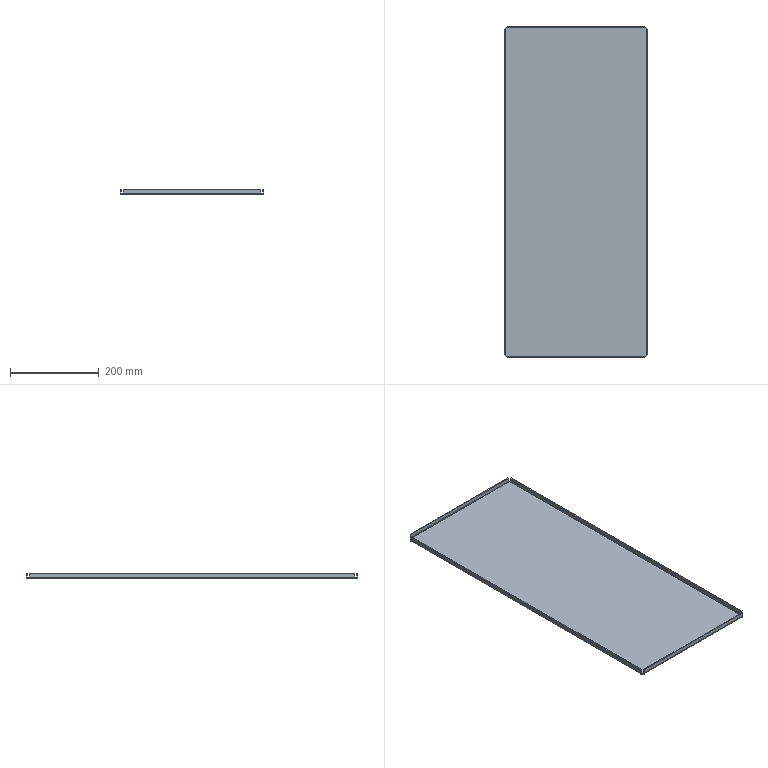Part | SolidWorks | features BaseBody 1 | 1 solid | 50 faces | box 325 x 750 x 12 mm | volume 654399 mm3 | plane 42 | cylinder 8 | commonest cylinder face diameters 1.473 x4 6.473 x4
STEP:
#1=CARTESIAN_POINT('',(-155.5,372.5,9.5));
#2=VERTEX_POINT('',#1);
#3=CARTESIAN_POINT('',(155.5,372.5,9.5));
#4=VERTEX_POINT('',#3);
#5=CARTESIAN_POINT('',(155.5,372.5,9.5));
#6=DIRECTION('',(1.,0.,0.));
#7=VECTOR('',#6,1000.);
#8=LINE('',#5,#7);
#9=EDGE_CURVE('',#2,#4,#8,.T.);
#10=ORIENTED_EDGE('',*,*,#9,.T.);
#11=CARTESIAN_POINT('',(155.5,375.,9.5));
#12=VERTEX_POINT('',#11);
#13=CARTESIAN_POINT('',(155.5,375.,9.5));
#14=DIRECTION('',(0.,-1.,0.));
#15=VECTOR('',#14,1000.);
#16=LINE('',#13,#15);
#17=EDGE_CURVE('',#12,#4,#16,.T.);
#18=ORIENTED_EDGE('',*,*,#17,.F.);
#19=CARTESIAN_POINT('',(-155.5,375.,9.5));
#20=VERTEX_POINT('',#19);
#21=CARTESIAN_POINT('',(0.,375.,9.5));
#22=DIRECTION('',(1.,0.,0.));
#23=VECTOR('',#22,1000.);
#24=LINE('',#21,#23);
#25=EDGE_CURVE('',#20,#12,#24,.T.);
#26=ORIENTED_EDGE('',*,*,#25,.F.);
#27=CARTESIAN_POINT('',(-155.5,375.,9.5));
#28=DIRECTION('',(0.,-1.,0.));
#29=VECTOR('',#28,1000.);
#30=LINE('',#27,#29);
#31=EDGE_CURVE('',#20,#2,#30,.T.);
#32=ORIENTED_EDGE('',*,*,#31,.T.);
#33=EDGE_LOOP('',(#10,#18,#26,#32));
#34=FACE_OUTER_BOUND('',#33,.T.);
#35=CARTESIAN_POINT('',(155.5,375.,9.5));
#36=DIRECTION('',(0.,0.,-1.));
#37=DIRECTION('',(0.,-1.,0.));
#38=AXIS2_PLACEMENT_3D('',#35,#36,#37);
#39=PLANE('',#38);
#40=ADVANCED_FACE('',(#34),#39,.F.);
#41=CARTESIAN_POINT('',(-155.5,372.5,0.7366));
#42=VERTEX_POINT('',#41);
#43=CARTESIAN_POINT('',(-155.5,372.5,9.5));
#44=DIRECTION('',(0.,0.,1.));
#45=VECTOR('',#44,1000.);
#46=LINE('',#43,#45);
#47=EDGE_CURVE('',#42,#2,#46,.T.);
#48=ORIENTED_EDGE('',*,*,#47,.F.);
#49=CARTESIAN_POINT('',(155.5,372.5,0.7366));
#50=VERTEX_POINT('',#49);
#51=CARTESIAN_POINT('',(155.5,372.5,0.7366));
#52=DIRECTION('',(-1.,0.,0.));
#53=VECTOR('',#52,1000.);
#54=LINE('',#51,#53);
#55=EDGE_CURVE('',#50,#42,#54,.T.);
#56=ORIENTED_EDGE('',*,*,#55,.F.);
#57=CARTESIAN_POINT('',(155.5,372.5,0.));
#58=DIRECTION('',(0.,0.,-1.));
#59=VECTOR('',#58,1000.);
#60=LINE('',#57,#59);
#61=EDGE_CURVE('',#4,#50,#60,.T.);
#62=ORIENTED_EDGE('',*,*,#61,.F.);
#63=ORIENTED_EDGE('',*,*,#9,.F.);
#64=EDGE_LOOP('',(#48,#56,#62,#63));
#65=FACE_OUTER_BOUND('',#64,.T.);
#66=CARTESIAN_POINT('',(0.,372.5,0.));
#67=DIRECTION('',(0.,-1.,0.));
#68=DIRECTION('',(-1.,0.,0.));
#69=AXIS2_PLACEMENT_3D('',#66,#67,#68);
#70=PLANE('',#69);
#71=ADVANCED_FACE('',(#65),#70,.T.);
#72=CARTESIAN_POINT('',(-155.5,375.,0.7366));
#73=VERTEX_POINT('',#72);
#74=CARTESIAN_POINT('',(155.5,375.,0.7366));
#75=VERTEX_POINT('',#74);
#76=CARTESIAN_POINT('',(155.5,375.,0.7366));
#77=DIRECTION('',(1.,0.,0.));
#78=VECTOR('',#77,1000.);
#79=LINE('',#76,#78);
#80=EDGE_CURVE('',#73,#75,#79,.T.);
#81=ORIENTED_EDGE('',*,*,#80,.F.);
#82=CARTESIAN_POINT('',(-155.5,375.,0.));
#83=DIRECTION('',(0.,0.,1.));
#84=VECTOR('',#83,1000.);
#85=LINE('',#82,#84);
#86=EDGE_CURVE('',#73,#20,#85,.T.);
#87=ORIENTED_EDGE('',*,*,#86,.T.);
#88=ORIENTED_EDGE('',*,*,#25,.T.);
#89=CARTESIAN_POINT('',(155.5,375.,0.));
#90=DIRECTION('',(0.,0.,-1.));
#91=VECTOR('',#90,1000.);
#92=LINE('',#89,#91);
#93=EDGE_CURVE('',#12,#75,#92,.T.);
#94=ORIENTED_EDGE('',*,*,#93,.T.);
#95=EDGE_LOOP('',(#81,#87,#88,#94));
#96=FACE_OUTER_BOUND('',#95,.T.);
#97=CARTESIAN_POINT('',(0.,375.,0.));
#98=DIRECTION('',(0.,-1.,0.));
#99=DIRECTION('',(-1.,0.,0.));
#100=AXIS2_PLACEMENT_3D('',#97,#98,#99);
#101=PLANE('',#100);
#102=ADVANCED_FACE('',(#96),#101,.F.);
#103=CARTESIAN_POINT('',(-155.5,372.5,0.7366));
#104=DIRECTION('',(0.,1.,0.));
#105=VECTOR('',#104,1000.);
#106=LINE('',#103,#105);
#107=EDGE_CURVE('',#42,#73,#106,.T.);
#108=ORIENTED_EDGE('',*,*,#107,.F.);
#109=ORIENTED_EDGE('',*,*,#47,.T.);
#110=ORIENTED_EDGE('',*,*,#31,.F.);
#111=ORIENTED_EDGE('',*,*,#86,.F.);
#112=EDGE_LOOP('',(#108,#109,#110,#111));
#113=FACE_OUTER_BOUND('',#112,.T.);
#114=CARTESIAN_POINT('',(-155.5,375.,9.5));
#115=DIRECTION('',(1.,0.,0.));
#116=DIRECTION('',(0.,0.,-1.));
#117=AXIS2_PLACEMENT_3D('',#114,#115,#116);
#118=PLANE('',#117);
#119=ADVANCED_FACE('',(#113),#118,.F.);
#120=CARTESIAN_POINT('',(155.5,375.,0.7366));
#121=DIRECTION('',(0.,1.,0.));
#122=VECTOR('',#121,1000.);
#123=LINE('',#120,#122);
#124=EDGE_CURVE('',#50,#75,#123,.T.);
#125=ORIENTED_EDGE('',*,*,#124,.T.);
#126=ORIENTED_EDGE('',*,*,#93,.F.);
#127=ORIENTED_EDGE('',*,*,#17,.T.);
#128=ORIENTED_EDGE('',*,*,#61,.T.);
#129=EDGE_LOOP('',(#125,#126,#127,#128));
#130=FACE_OUTER_BOUND('',#129,.T.);
#131=CARTESIAN_POINT('',(155.5,375.,0.));
#132=DIRECTION('',(-1.,0.,0.));
#133=DIRECTION('',(0.,1.,0.));
#134=AXIS2_PLACEMENT_3D('',#131,#132,#133);
#135=PLANE('',#134);
#136=ADVANCED_FACE('',(#130),#135,.F.);
#137=CARTESIAN_POINT('',(-155.5,371.763,0.));
#138=VERTEX_POINT('',#137);
#139=CARTESIAN_POINT('',(155.5,371.763,0.));
#140=VERTEX_POINT('',#139);
#141=CARTESIAN_POINT('',(-155.5,371.763,0.));
#142=DIRECTION('',(1.,0.,0.));
#143=VECTOR('',#142,1000.);
#144=LINE('',#141,#143);
#145=EDGE_CURVE('',#138,#140,#144,.T.);
#146=ORIENTED_EDGE('',*,*,#145,.T.);
#147=CARTESIAN_POINT('',(155.5,371.763,0.7366));
#148=DIRECTION('',(1.,0.,0.));
#149=DIRECTION('',(0.,0.,1.));
#150=AXIS2_PLACEMENT_3D('',#147,#148,#149);
#151=CIRCLE('',#150,0.7366);
#152=EDGE_CURVE('',#140,#50,#151,.T.);
#153=ORIENTED_EDGE('',*,*,#152,.T.);
#154=ORIENTED_EDGE('',*,*,#55,.T.);
#155=CARTESIAN_POINT('',(-155.5,371.763,0.7366));
#156=DIRECTION('',(-1.,0.,0.));
#157=DIRECTION('',(0.,0.,1.));
#158=AXIS2_PLACEMENT_3D('',#155,#156,#157);
#159=CIRCLE('',#158,0.7366);
#160=EDGE_CURVE('',#42,#138,#159,.T.);
#161=ORIENTED_EDGE('',*,*,#160,.T.);
#162=EDGE_LOOP('',(#146,#153,#154,#161));
#163=FACE_OUTER_BOUND('',#162,.T.);
#164=CARTESIAN_POINT('',(-155.5,371.763,0.7366));
#165=DIRECTION('',(-1.,0.,0.));
#166=DIRECTION('',(0.,1.,0.));
#167=AXIS2_PLACEMENT_3D('',#164,#165,#166);
#168=CYLINDRICAL_SURFACE('',#167,0.7366);
#169=ADVANCED_FACE('',(#163),#168,.F.);
#170=CARTESIAN_POINT('',(-155.5,371.763,-2.5));
#171=VERTEX_POINT('',#170);
#172=CARTESIAN_POINT('',(155.5,371.763,-2.5));
#173=VERTEX_POINT('',#172);
#174=CARTESIAN_POINT('',(-155.5,371.763,-2.5));
#175=DIRECTION('',(1.,0.,0.));
#176=VECTOR('',#175,1000.);
#177=LINE('',#174,#176);
#178=EDGE_CURVE('',#171,#173,#177,.T.);
#179=ORIENTED_EDGE('',*,*,#178,.F.);
#180=CARTESIAN_POINT('',(-155.5,374.915,0.));
#181=VERTEX_POINT('',#180);
#182=CARTESIAN_POINT('',(-155.5,371.763,0.7366));
#183=DIRECTION('',(-1.,0.,0.));
#184=DIRECTION('',(0.,0.,1.));
#185=AXIS2_PLACEMENT_3D('',#182,#183,#184);
#186=CIRCLE('',#185,3.237);
#187=EDGE_CURVE('',#181,#171,#186,.T.);
#188=ORIENTED_EDGE('',*,*,#187,.F.);
#189=CARTESIAN_POINT('',(-155.5,371.763,0.7366));
#190=DIRECTION('',(-1.,0.,0.));
#191=DIRECTION('',(0.,0.,1.));
#192=AXIS2_PLACEMENT_3D('',#189,#190,#191);
#193=CIRCLE('',#192,3.237);
#194=EDGE_CURVE('',#73,#181,#193,.T.);
#195=ORIENTED_EDGE('',*,*,#194,.F.);
#196=ORIENTED_EDGE('',*,*,#80,.T.);
#197=CARTESIAN_POINT('',(155.5,374.915,0.));
#198=VERTEX_POINT('',#197);
#199=CARTESIAN_POINT('',(155.5,371.763,0.7366));
#200=DIRECTION('',(1.,0.,0.));
#201=DIRECTION('',(0.,0.,1.));
#202=AXIS2_PLACEMENT_3D('',#199,#200,#201);
#203=CIRCLE('',#202,3.237);
#204=EDGE_CURVE('',#198,#75,#203,.T.);
#205=ORIENTED_EDGE('',*,*,#204,.F.);
#206=CARTESIAN_POINT('',(155.5,371.763,0.7366));
#207=DIRECTION('',(1.,0.,0.));
#208=DIRECTION('',(0.,0.,1.));
#209=AXIS2_PLACEMENT_3D('',#206,#207,#208);
#210=CIRCLE('',#209,3.237);
#211=EDGE_CURVE('',#173,#198,#210,.T.);
#212=ORIENTED_EDGE('',*,*,#211,.F.);
#213=EDGE_LOOP('',(#179,#188,#195,#196,#205,#212));
#214=FACE_OUTER_BOUND('',#213,.T.);
#215=CARTESIAN_POINT('',(-155.5,371.763,0.7366));
#216=DIRECTION('',(-1.,0.,0.));
#217=DIRECTION('',(0.,1.,0.));
#218=AXIS2_PLACEMENT_3D('',#215,#216,#217);
#219=CYLINDRICAL_SURFACE('',#218,3.237);
#220=ADVANCED_FACE('',(#214),#219,.T.);
#221=ORIENTED_EDGE('',*,*,#194,.T.);
#222=CARTESIAN_POINT('',(-155.5,375.,0.));
#223=DIRECTION('',(0.,-1.,0.));
#224=VECTOR('',#223,1000.);
#225=LINE('',#222,#224);
#226=EDGE_CURVE('',#181,#138,#225,.T.);
#227=ORIENTED_EDGE('',*,*,#226,.T.);
#228=ORIENTED_EDGE('',*,*,#160,.F.);
#229=ORIENTED_EDGE('',*,*,#107,.T.);
#230=EDGE_LOOP('',(#221,#227,#228,#229));
#231=FACE_OUTER_BOUND('',#230,.T.);
#232=CARTESIAN_POINT('',(-155.5,371.763,0.7366));
#233=DIRECTION('',(1.,0.,0.));
#234=DIRECTION('',(0.,1.,0.));
#235=AXIS2_PLACEMENT_3D('',#232,#233,#234);
#236=PLANE('',#235);
#237=ADVANCED_FACE('',(#231),#236,.F.);
#238=ORIENTED_EDGE('',*,*,#152,.F.);
#239=CARTESIAN_POINT('',(155.5,371.763,0.));
#240=DIRECTION('',(0.,1.,0.));
#241=VECTOR('',#240,1000.);
#242=LINE('',#239,#241);
#243=EDGE_CURVE('',#140,#198,#242,.T.);
#244=ORIENTED_EDGE('',*,*,#243,.T.);
#245=ORIENTED_EDGE('',*,*,#204,.T.);
#246=ORIENTED_EDGE('',*,*,#124,.F.);
#247=EDGE_LOOP('',(#238,#244,#245,#246));
#248=FACE_OUTER_BOUND('',#247,.T.);
#249=CARTESIAN_POINT('',(155.5,371.763,0.7366));
#250=DIRECTION('',(1.,0.,0.));
#251=DIRECTION('',(0.,1.,0.));
#252=AXIS2_PLACEMENT_3D('',#249,#250,#251);
#253=PLANE('',#252);
#254=ADVANCED_FACE('',(#248),#253,.T.);
#255=CARTESIAN_POINT('',(160.,368.,9.5));
#256=VERTEX_POINT('',#255);
#257=CARTESIAN_POINT('',(160.,-368.,9.5));
#258=VERTEX_POINT('',#257);
#259=CARTESIAN_POINT('',(160.,-368.,9.5));
#260=DIRECTION('',(0.,-1.,0.));
#261=VECTOR('',#260,1000.);
#262=LINE('',#259,#261);
#263=EDGE_CURVE('',#256,#258,#262,.T.);
#264=ORIENTED_EDGE('',*,*,#263,.T.);
#265=CARTESIAN_POINT('',(162.5,-368.,9.5));
#266=VERTEX_POINT('',#265);
#267=CARTESIAN_POINT('',(162.5,-368.,9.5));
#268=DIRECTION('',(-1.,0.,0.));
#269=VECTOR('',#268,1000.);
#270=LINE('',#267,#269);
#271=EDGE_CURVE('',#266,#258,#270,.T.);
#272=ORIENTED_EDGE('',*,*,#271,.F.);
#273=CARTESIAN_POINT('',(162.5,368.,9.5));
#274=VERTEX_POINT('',#273);
#275=CARTESIAN_POINT('',(162.5,0.,9.5));
#276=DIRECTION('',(0.,-1.,0.));
#277=VECTOR('',#276,1000.);
#278=LINE('',#275,#277);
#279=EDGE_CURVE('',#274,#266,#278,.T.);
#280=ORIENTED_EDGE('',*,*,#279,.F.);
#281=CARTESIAN_POINT('',(162.5,368.,9.5));
#282=DIRECTION('',(-1.,0.,0.));
#283=VECTOR('',#282,1000.);
#284=LINE('',#281,#283);
#285=EDGE_CURVE('',#274,#256,#284,.T.);
#286=ORIENTED_EDGE('',*,*,#285,.T.);
#287=EDGE_LOOP('',(#264,#272,#280,#286));
#288=FACE_OUTER_BOUND('',#287,.T.);
#289=CARTESIAN_POINT('',(162.5,-368.,9.5));
#290=DIRECTION('',(0.,0.,-1.));
#291=DIRECTION('',(-1.,0.,0.));
#292=AXIS2_PLACEMENT_3D('',#289,#290,#291);
#293=PLANE('',#292);
#294=ADVANCED_FACE('',(#288),#293,.F.);
#295=CARTESIAN_POINT('',(160.,368.,0.7366));
#296=VERTEX_POINT('',#295);
#297=CARTESIAN_POINT('',(160.,368.,9.5));
#298=DIRECTION('',(0.,0.,1.));
#299=VECTOR('',#298,1000.);
#300=LINE('',#297,#299);
#301=EDGE_CURVE('',#296,#256,#300,.T.);
#302=ORIENTED_EDGE('',*,*,#301,.F.);
#303=CARTESIAN_POINT('',(160.,-368.,0.7366));
#304=VERTEX_POINT('',#303);
#305=CARTESIAN_POINT('',(160.,-368.,0.7366));
#306=DIRECTION('',(0.,1.,0.));
#307=VECTOR('',#306,1000.);
#308=LINE('',#305,#307);
#309=EDGE_CURVE('',#304,#296,#308,.T.);
#310=ORIENTED_EDGE('',*,*,#309,.F.);
#311=CARTESIAN_POINT('',(160.,-368.,0.));
#312=DIRECTION('',(0.,0.,-1.));
#313=VECTOR('',#312,1000.);
#314=LINE('',#311,#313);
#315=EDGE_CURVE('',#258,#304,#314,.T.);
#316=ORIENTED_EDGE('',*,*,#315,.F.);
#317=ORIENTED_EDGE('',*,*,#263,.F.);
#318=EDGE_LOOP('',(#302,#310,#316,#317));
#319=FACE_OUTER_BOUND('',#318,.T.);
#320=CARTESIAN_POINT('',(160.,0.,0.));
#321=DIRECTION('',(-1.,0.,0.));
#322=DIRECTION('',(0.,1.,0.));
#323=AXIS2_PLACEMENT_3D('',#320,#321,#322);
#324=PLANE('',#323);
#325=ADVANCED_FACE('',(#319),#324,.T.);
#326=CARTESIAN_POINT('',(162.5,368.,0.7366));
#327=VERTEX_POINT('',#326);
#328=CARTESIAN_POINT('',(162.5,-368.,0.7366));
#329=VERTEX_POINT('',#328);
#330=CARTESIAN_POINT('',(162.5,-368.,0.7366));
#331=DIRECTION('',(0.,-1.,0.));
#332=VECTOR('',#331,1000.);
#333=LINE('',#330,#332);
#334=EDGE_CURVE('',#327,#329,#333,.T.);
#335=ORIENTED_EDGE('',*,*,#334,.F.);
#336=CARTESIAN_POINT('',(162.5,368.,0.));
#337=DIRECTION('',(0.,0.,1.));
#338=VECTOR('',#337,1000.);
#339=LINE('',#336,#338);
#340=EDGE_CURVE('',#327,#274,#339,.T.);
#341=ORIENTED_EDGE('',*,*,#340,.T.);
#342=ORIENTED_EDGE('',*,*,#279,.T.);
#343=CARTESIAN_POINT('',(162.5,-368.,0.));
#344=DIRECTION('',(0.,0.,-1.));
#345=VECTOR('',#344,1000.);
#346=LINE('',#343,#345);
#347=EDGE_CURVE('',#266,#329,#346,.T.);
#348=ORIENTED_EDGE('',*,*,#347,.T.);
#349=EDGE_LOOP('',(#335,#341,#342,#348));
#350=FACE_OUTER_BOUND('',#349,.T.);
#351=CARTESIAN_POINT('',(162.5,0.,0.));
#352=DIRECTION('',(-1.,0.,0.));
#353=DIRECTION('',(0.,1.,0.));
#354=AXIS2_PLACEMENT_3D('',#351,#352,#353);
#355=PLANE('',#354);
#356=ADVANCED_FACE('',(#350),#355,.F.);
#357=CARTESIAN_POINT('',(160.,368.,0.7366));
#358=DIRECTION('',(1.,0.,0.));
#359=VECTOR('',#358,1000.);
#360=LINE('',#357,#359);
#361=EDGE_CURVE('',#296,#327,#360,.T.);
#362=ORIENTED_EDGE('',*,*,#361,.F.);
#363=ORIENTED_EDGE('',*,*,#301,.T.);
#364=ORIENTED_EDGE('',*,*,#285,.F.);
#365=ORIENTED_EDGE('',*,*,#340,.F.);
#366=EDGE_LOOP('',(#362,#363,#364,#365));
#367=FACE_OUTER_BOUND('',#366,.T.);
#368=CARTESIAN_POINT('',(162.5,368.,9.5));
#369=DIRECTION('',(0.,-1.,0.));
#370=DIRECTION('',(0.,0.,-1.));
#371=AXIS2_PLACEMENT_3D('',#368,#369,#370);
#372=PLANE('',#371);
#373=ADVANCED_FACE('',(#367),#372,.F.);
#374=CARTESIAN_POINT('',(162.5,-368.,0.7366));
#375=DIRECTION('',(1.,0.,0.));
#376=VECTOR('',#375,1000.);
#377=LINE('',#374,#376);
#378=EDGE_CURVE('',#304,#329,#377,.T.);
#379=ORIENTED_EDGE('',*,*,#378,.T.);
#380=ORIENTED_EDGE('',*,*,#347,.F.);
#381=ORIENTED_EDGE('',*,*,#271,.T.);
#382=ORIENTED_EDGE('',*,*,#315,.T.);
#383=EDGE_LOOP('',(#379,#380,#381,#382));
#384=FACE_OUTER_BOUND('',#383,.T.);
#385=CARTESIAN_POINT('',(162.5,-368.,0.));
#386=DIRECTION('',(0.,1.,0.));
#387=DIRECTION('',(1.,0.,0.));
#388=AXIS2_PLACEMENT_3D('',#385,#386,#387);
#389=PLANE('',#388);
#390=ADVANCED_FACE('',(#384),#389,.F.);
#391=CARTESIAN_POINT('',(159.263,368.,0.));
#392=VERTEX_POINT('',#391);
#393=CARTESIAN_POINT('',(159.263,-368.,0.));
#394=VERTEX_POINT('',#393);
#395=CARTESIAN_POINT('',(159.263,368.,0.));
#396=DIRECTION('',(0.,-1.,0.));
#397=VECTOR('',#396,1000.);
#398=LINE('',#395,#397);
#399=EDGE_CURVE('',#392,#394,#398,.T.);
#400=ORIENTED_EDGE('',*,*,#399,.T.);
#401=CARTESIAN_POINT('',(159.263,-368.,0.7366));
#402=DIRECTION('',(0.,-1.,0.));
#403=DIRECTION('',(0.,0.,1.));
#404=AXIS2_PLACEMENT_3D('',#401,#402,#403);
#405=CIRCLE('',#404,0.7366);
#406=EDGE_CURVE('',#394,#304,#405,.T.);
#407=ORIENTED_EDGE('',*,*,#406,.T.);
#408=ORIENTED_EDGE('',*,*,#309,.T.);
#409=CARTESIAN_POINT('',(159.263,368.,0.7366));
#410=DIRECTION('',(0.,1.,0.));
#411=DIRECTION('',(0.,0.,1.));
#412=AXIS2_PLACEMENT_3D('',#409,#410,#411);
#413=CIRCLE('',#412,0.7366);
#414=EDGE_CURVE('',#296,#392,#413,.T.);
#415=ORIENTED_EDGE('',*,*,#414,.T.);
#416=EDGE_LOOP('',(#400,#407,#408,#415));
#417=FACE_OUTER_BOUND('',#416,.T.);
#418=CARTESIAN_POINT('',(159.263,368.,0.7366));
#419=DIRECTION('',(0.,1.,0.));
#420=DIRECTION('',(1.,0.,0.));
#421=AXIS2_PLACEMENT_3D('',#418,#419,#420);
#422=CYLINDRICAL_SURFACE('',#421,0.7366);
#423=ADVANCED_FACE('',(#417),#422,.F.);
#424=CARTESIAN_POINT('',(159.263,368.,-2.5));
#425=VERTEX_POINT('',#424);
#426=CARTESIAN_POINT('',(159.263,-368.,-2.5));
#427=VERTEX_POINT('',#426);
#428=CARTESIAN_POINT('',(159.263,368.,-2.5));
#429=DIRECTION('',(0.,-1.,0.));
#430=VECTOR('',#429,1000.);
#431=LINE('',#428,#430);
#432=EDGE_CURVE('',#425,#427,#431,.T.);
#433=ORIENTED_EDGE('',*,*,#432,.F.);
#434=CARTESIAN_POINT('',(162.415,368.,0.));
#435=VERTEX_POINT('',#434);
#436=CARTESIAN_POINT('',(159.263,368.,0.7366));
#437=DIRECTION('',(0.,1.,0.));
#438=DIRECTION('',(0.,0.,1.));
#439=AXIS2_PLACEMENT_3D('',#436,#437,#438);
#440=CIRCLE('',#439,3.237);
#441=EDGE_CURVE('',#435,#425,#440,.T.);
#442=ORIENTED_EDGE('',*,*,#441,.F.);
#443=CARTESIAN_POINT('',(159.263,368.,0.7366));
#444=DIRECTION('',(0.,1.,0.));
#445=DIRECTION('',(0.,0.,1.));
#446=AXIS2_PLACEMENT_3D('',#443,#444,#445);
#447=CIRCLE('',#446,3.237);
#448=EDGE_CURVE('',#327,#435,#447,.T.);
#449=ORIENTED_EDGE('',*,*,#448,.F.);
#450=ORIENTED_EDGE('',*,*,#334,.T.);
#451=CARTESIAN_POINT('',(162.415,-368.,0.));
#452=VERTEX_POINT('',#451);
#453=CARTESIAN_POINT('',(159.263,-368.,0.7366));
#454=DIRECTION('',(0.,-1.,0.));
#455=DIRECTION('',(0.,0.,1.));
#456=AXIS2_PLACEMENT_3D('',#453,#454,#455);
#457=CIRCLE('',#456,3.237);
#458=EDGE_CURVE('',#452,#329,#457,.T.);
#459=ORIENTED_EDGE('',*,*,#458,.F.);
#460=CARTESIAN_POINT('',(159.263,-368.,0.7366));
#461=DIRECTION('',(0.,-1.,0.));
#462=DIRECTION('',(0.,0.,1.));
#463=AXIS2_PLACEMENT_3D('',#460,#461,#462);
#464=CIRCLE('',#463,3.237);
#465=EDGE_CURVE('',#427,#452,#464,.T.);
#466=ORIENTED_EDGE('',*,*,#465,.F.);
#467=EDGE_LOOP('',(#433,#442,#449,#450,#459,#466));
#468=FACE_OUTER_BOUND('',#467,.T.);
#469=CARTESIAN_POINT('',(159.263,368.,0.7366));
#470=DIRECTION('',(0.,1.,0.));
#471=DIRECTION('',(1.,0.,0.));
#472=AXIS2_PLACEMENT_3D('',#469,#470,#471);
#473=CYLINDRICAL_SURFACE('',#472,3.237);
#474=ADVANCED_FACE('',(#468),#473,.T.);
#475=ORIENTED_EDGE('',*,*,#448,.T.);
#476=CARTESIAN_POINT('',(162.5,368.,0.));
#477=DIRECTION('',(-1.,0.,0.));
#478=VECTOR('',#477,1000.);
#479=LINE('',#476,#478);
#480=EDGE_CURVE('',#435,#392,#479,.T.);
#481=ORIENTED_EDGE('',*,*,#480,.T.);
#482=ORIENTED_EDGE('',*,*,#414,.F.);
#483=ORIENTED_EDGE('',*,*,#361,.T.);
#484=EDGE_LOOP('',(#475,#481,#482,#483));
#485=FACE_OUTER_BOUND('',#484,.T.);
#486=CARTESIAN_POINT('',(159.263,368.,0.7366));
#487=DIRECTION('',(0.,-1.,0.));
#488=DIRECTION('',(0.,0.,-1.));
#489=AXIS2_PLACEMENT_3D('',#486,#487,#488);
#490=PLANE('',#489);
#491=ADVANCED_FACE('',(#485),#490,.F.);
#492=ORIENTED_EDGE('',*,*,#406,.F.);
#493=CARTESIAN_POINT('',(159.263,-368.,0.));
#494=DIRECTION('',(1.,0.,0.));
#495=VECTOR('',#494,1000.);
#496=LINE('',#493,#495);
#497=EDGE_CURVE('',#394,#452,#496,.T.);
#498=ORIENTED_EDGE('',*,*,#497,.T.);
#499=ORIENTED_EDGE('',*,*,#458,.T.);
#500=ORIENTED_EDGE('',*,*,#378,.F.);
#501=EDGE_LOOP('',(#492,#498,#499,#500));
#502=FACE_OUTER_BOUND('',#501,.T.);
#503=CARTESIAN_POINT('',(159.263,-368.,0.7366));
#504=DIRECTION('',(0.,-1.,0.));
#505=DIRECTION('',(0.,0.,-1.));
#506=AXIS2_PLACEMENT_3D('',#503,#504,#505);
#507=PLANE('',#506);
#508=ADVANCED_FACE('',(#502),#507,.T.);
#509=CARTESIAN_POINT('',(155.5,-372.5,9.5));
#510=VERTEX_POINT('',#509);
#511=CARTESIAN_POINT('',(-155.5,-372.5,9.5));
#512=VERTEX_POINT('',#511);
#513=CARTESIAN_POINT('',(-155.5,-372.5,9.5));
#514=DIRECTION('',(-1.,0.,0.));
#515=VECTOR('',#514,1000.);
#516=LINE('',#513,#515);
#517=EDGE_CURVE('',#510,#512,#516,.T.);
#518=ORIENTED_EDGE('',*,*,#517,.T.);
#519=CARTESIAN_POINT('',(-155.5,-375.,9.5));
#520=VERTEX_POINT('',#519);
#521=CARTESIAN_POINT('',(-155.5,-375.,9.5));
#522=DIRECTION('',(0.,1.,0.));
#523=VECTOR('',#522,1000.);
#524=LINE('',#521,#523);
#525=EDGE_CURVE('',#520,#512,#524,.T.);
#526=ORIENTED_EDGE('',*,*,#525,.F.);
#527=CARTESIAN_POINT('',(155.5,-375.,9.5));
#528=VERTEX_POINT('',#527);
#529=CARTESIAN_POINT('',(0.,-375.,9.5));
#530=DIRECTION('',(-1.,0.,0.));
#531=VECTOR('',#530,1000.);
#532=LINE('',#529,#531);
#533=EDGE_CURVE('',#528,#520,#532,.T.);
#534=ORIENTED_EDGE('',*,*,#533,.F.);
#535=CARTESIAN_POINT('',(155.5,-375.,9.5));
#536=DIRECTION('',(0.,1.,0.));
#537=VECTOR('',#536,1000.);
#538=LINE('',#535,#537);
#539=EDGE_CURVE('',#528,#510,#538,.T.);
#540=ORIENTED_EDGE('',*,*,#539,.T.);
#541=EDGE_LOOP('',(#518,#526,#534,#540));
#542=FACE_OUTER_BOUND('',#541,.T.);
#543=CARTESIAN_POINT('',(-155.5,-375.,9.5));
#544=DIRECTION('',(0.,0.,-1.));
#545=DIRECTION('',(-1.,0.,0.));
#546=AXIS2_PLACEMENT_3D('',#543,#544,#545);
#547=PLANE('',#546);
#548=ADVANCED_FACE('',(#542),#547,.F.);
#549=CARTESIAN_POINT('',(155.5,-372.5,0.7366));
#550=VERTEX_POINT('',#549);
#551=CARTESIAN_POINT('',(155.5,-372.5,9.5));
#552=DIRECTION('',(0.,0.,1.));
#553=VECTOR('',#552,1000.);
#554=LINE('',#551,#553);
#555=EDGE_CURVE('',#550,#510,#554,.T.);
#556=ORIENTED_EDGE('',*,*,#555,.F.);
#557=CARTESIAN_POINT('',(-155.5,-372.5,0.7366));
#558=VERTEX_POINT('',#557);
#559=CARTESIAN_POINT('',(-155.5,-372.5,0.7366));
#560=DIRECTION('',(1.,0.,0.));
#561=VECTOR('',#560,1000.);
#562=LINE('',#559,#561);
#563=EDGE_CURVE('',#558,#550,#562,.T.);
#564=ORIENTED_EDGE('',*,*,#563,.F.);
#565=CARTESIAN_POINT('',(-155.5,-372.5,0.));
#566=DIRECTION('',(0.,0.,-1.));
#567=VECTOR('',#566,1000.);
#568=LINE('',#565,#567);
#569=EDGE_CURVE('',#512,#558,#568,.T.);
#570=ORIENTED_EDGE('',*,*,#569,.F.);
#571=ORIENTED_EDGE('',*,*,#517,.F.);
#572=EDGE_LOOP('',(#556,#564,#570,#571));
#573=FACE_OUTER_BOUND('',#572,.T.);
#574=CARTESIAN_POINT('',(0.,-372.5,0.));
#575=DIRECTION('',(0.,1.,0.));
#576=DIRECTION('',(0.,0.,-1.));
#577=AXIS2_PLACEMENT_3D('',#574,#575,#576);
#578=PLANE('',#577);
#579=ADVANCED_FACE('',(#573),#578,.T.);
#580=CARTESIAN_POINT('',(155.5,-375.,0.7366));
#581=VERTEX_POINT('',#580);
#582=CARTESIAN_POINT('',(-155.5,-375.,0.7366));
#583=VERTEX_POINT('',#582);
#584=CARTESIAN_POINT('',(-155.5,-375.,0.7366));
#585=DIRECTION('',(-1.,0.,0.));
#586=VECTOR('',#585,1000.);
#587=LINE('',#584,#586);
#588=EDGE_CURVE('',#581,#583,#587,.T.);
#589=ORIENTED_EDGE('',*,*,#588,.F.);
#590=CARTESIAN_POINT('',(155.5,-375.,0.));
#591=DIRECTION('',(0.,0.,1.));
#592=VECTOR('',#591,1000.);
#593=LINE('',#590,#592);
#594=EDGE_CURVE('',#581,#528,#593,.T.);
#595=ORIENTED_EDGE('',*,*,#594,.T.);
#596=ORIENTED_EDGE('',*,*,#533,.T.);
#597=CARTESIAN_POINT('',(-155.5,-375.,0.));
#598=DIRECTION('',(0.,0.,-1.));
#599=VECTOR('',#598,1000.);
#600=LINE('',#597,#599);
#601=EDGE_CURVE('',#520,#583,#600,.T.);
#602=ORIENTED_EDGE('',*,*,#601,.T.);
#603=EDGE_LOOP('',(#589,#595,#596,#602));
#604=FACE_OUTER_BOUND('',#603,.T.);
#605=CARTESIAN_POINT('',(0.,-375.,0.));
#606=DIRECTION('',(0.,1.,0.));
#607=DIRECTION('',(0.,0.,-1.));
#608=AXIS2_PLACEMENT_3D('',#605,#606,#607);
#609=PLANE('',#608);
#610=ADVANCED_FACE('',(#604),#609,.F.);
#611=CARTESIAN_POINT('',(155.5,-372.5,0.7366));
#612=DIRECTION('',(0.,-1.,0.));
#613=VECTOR('',#612,1000.);
#614=LINE('',#611,#613);
#615=EDGE_CURVE('',#550,#581,#614,.T.);
#616=ORIENTED_EDGE('',*,*,#615,.F.);
#617=ORIENTED_EDGE('',*,*,#555,.T.);
#618=ORIENTED_EDGE('',*,*,#539,.F.);
#619=ORIENTED_EDGE('',*,*,#594,.F.);
#620=EDGE_LOOP('',(#616,#617,#618,#619));
#621=FACE_OUTER_BOUND('',#620,.T.);
#622=CARTESIAN_POINT('',(155.5,-375.,9.5));
#623=DIRECTION('',(-1.,0.,0.));
#624=DIRECTION('',(0.,1.,0.));
#625=AXIS2_PLACEMENT_3D('',#622,#623,#624);
#626=PLANE('',#625);
#627=ADVANCED_FACE('',(#621),#626,.F.);
#628=CARTESIAN_POINT('',(-155.5,-375.,0.7366));
#629=DIRECTION('',(0.,-1.,0.));
#630=VECTOR('',#629,1000.);
#631=LINE('',#628,#630);
#632=EDGE_CURVE('',#558,#583,#631,.T.);
#633=ORIENTED_EDGE('',*,*,#632,.T.);
#634=ORIENTED_EDGE('',*,*,#601,.F.);
#635=ORIENTED_EDGE('',*,*,#525,.T.);
#636=ORIENTED_EDGE('',*,*,#569,.T.);
#637=EDGE_LOOP('',(#633,#634,#635,#636));
#638=FACE_OUTER_BOUND('',#637,.T.);
#639=CARTESIAN_POINT('',(-155.5,-375.,0.));
#640=DIRECTION('',(1.,0.,0.));
#641=DIRECTION('',(0.,0.,-1.));
#642=AXIS2_PLACEMENT_3D('',#639,#640,#641);
#643=PLANE('',#642);
#644=ADVANCED_FACE('',(#638),#643,.F.);
#645=CARTESIAN_POINT('',(155.5,-371.763,0.));
#646=VERTEX_POINT('',#645);
#647=CARTESIAN_POINT('',(-155.5,-371.763,0.));
#648=VERTEX_POINT('',#647);
#649=CARTESIAN_POINT('',(155.5,-371.763,0.));
#650=DIRECTION('',(-1.,0.,0.));
#651=VECTOR('',#650,1000.);
#652=LINE('',#649,#651);
#653=EDGE_CURVE('',#646,#648,#652,.T.);
#654=ORIENTED_EDGE('',*,*,#653,.T.);
#655=CARTESIAN_POINT('',(-155.5,-371.763,0.7366));
#656=DIRECTION('',(-1.,0.,0.));
#657=DIRECTION('',(0.,0.,-1.));
#658=AXIS2_PLACEMENT_3D('',#655,#656,#657);
#659=CIRCLE('',#658,0.7366);
#660=EDGE_CURVE('',#648,#558,#659,.T.);
#661=ORIENTED_EDGE('',*,*,#660,.T.);
#662=ORIENTED_EDGE('',*,*,#563,.T.);
#663=CARTESIAN_POINT('',(155.5,-371.763,0.7366));
#664=DIRECTION('',(1.,0.,0.));
#665=DIRECTION('',(0.,0.,-1.));
#666=AXIS2_PLACEMENT_3D('',#663,#664,#665);
#667=CIRCLE('',#666,0.7366);
#668=EDGE_CURVE('',#550,#646,#667,.T.);
#669=ORIENTED_EDGE('',*,*,#668,.T.);
#670=EDGE_LOOP('',(#654,#661,#662,#669));
#671=FACE_OUTER_BOUND('',#670,.T.);
#672=CARTESIAN_POINT('',(155.5,-371.763,0.7366));
#673=DIRECTION('',(1.,0.,0.));
#674=DIRECTION('',(0.,-1.,0.));
#675=AXIS2_PLACEMENT_3D('',#672,#673,#674);
#676=CYLINDRICAL_SURFACE('',#675,0.7366);
#677=ADVANCED_FACE('',(#671),#676,.F.);
#678=CARTESIAN_POINT('',(155.5,-371.763,-2.5));
#679=VERTEX_POINT('',#678);
#680=CARTESIAN_POINT('',(-155.5,-371.763,-2.5));
#681=VERTEX_POINT('',#680);
#682=CARTESIAN_POINT('',(155.5,-371.763,-2.5));
#683=DIRECTION('',(-1.,0.,0.));
#684=VECTOR('',#683,1000.);
#685=LINE('',#682,#684);
#686=EDGE_CURVE('',#679,#681,#685,.T.);
#687=ORIENTED_EDGE('',*,*,#686,.F.);
#688=CARTESIAN_POINT('',(155.5,-374.915,0.));
#689=VERTEX_POINT('',#688);
#690=CARTESIAN_POINT('',(155.5,-371.763,0.7366));
#691=DIRECTION('',(1.,0.,0.));
#692=DIRECTION('',(0.,0.,-1.));
#693=AXIS2_PLACEMENT_3D('',#690,#691,#692);
#694=CIRCLE('',#693,3.237);
#695=EDGE_CURVE('',#689,#679,#694,.T.);
#696=ORIENTED_EDGE('',*,*,#695,.F.);
#697=CARTESIAN_POINT('',(155.5,-371.763,0.7366));
#698=DIRECTION('',(1.,0.,0.));
#699=DIRECTION('',(0.,0.,-1.));
#700=AXIS2_PLACEMENT_3D('',#697,#698,#699);
#701=CIRCLE('',#700,3.237);
#702=EDGE_CURVE('',#581,#689,#701,.T.);
#703=ORIENTED_EDGE('',*,*,#702,.F.);
#704=ORIENTED_EDGE('',*,*,#588,.T.);
#705=CARTESIAN_POINT('',(-155.5,-374.915,0.));
#706=VERTEX_POINT('',#705);
#707=CARTESIAN_POINT('',(-155.5,-371.763,0.7366));
#708=DIRECTION('',(-1.,0.,0.));
#709=DIRECTION('',(0.,0.,-1.));
#710=AXIS2_PLACEMENT_3D('',#707,#708,#709);
#711=CIRCLE('',#710,3.237);
#712=EDGE_CURVE('',#706,#583,#711,.T.);
#713=ORIENTED_EDGE('',*,*,#712,.F.);
#714=CARTESIAN_POINT('',(-155.5,-371.763,0.7366));
#715=DIRECTION('',(-1.,0.,0.));
#716=DIRECTION('',(0.,0.,-1.));
#717=AXIS2_PLACEMENT_3D('',#714,#715,#716);
#718=CIRCLE('',#717,3.237);
#719=EDGE_CURVE('',#681,#706,#718,.T.);
#720=ORIENTED_EDGE('',*,*,#719,.F.);
#721=EDGE_LOOP('',(#687,#696,#703,#704,#713,#720));
#722=FACE_OUTER_BOUND('',#721,.T.);
#723=CARTESIAN_POINT('',(155.5,-371.763,0.7366));
#724=DIRECTION('',(1.,0.,0.));
#725=DIRECTION('',(0.,-1.,0.));
#726=AXIS2_PLACEMENT_3D('',#723,#724,#725);
#727=CYLINDRICAL_SURFACE('',#726,3.237);
#728=ADVANCED_FACE('',(#722),#727,.T.);
#729=ORIENTED_EDGE('',*,*,#702,.T.);
#730=CARTESIAN_POINT('',(155.5,-375.,0.));
#731=DIRECTION('',(0.,1.,0.));
#732=VECTOR('',#731,1000.);
#733=LINE('',#730,#732);
#734=EDGE_CURVE('',#689,#646,#733,.T.);
#735=ORIENTED_EDGE('',*,*,#734,.T.);
#736=ORIENTED_EDGE('',*,*,#668,.F.);
#737=ORIENTED_EDGE('',*,*,#615,.T.);
#738=EDGE_LOOP('',(#729,#735,#736,#737));
#739=FACE_OUTER_BOUND('',#738,.T.);
#740=CARTESIAN_POINT('',(155.5,-371.763,0.7366));
#741=DIRECTION('',(-1.,0.,0.));
#742=DIRECTION('',(0.,0.,1.));
#743=AXIS2_PLACEMENT_3D('',#740,#741,#742);
#744=PLANE('',#743);
#745=ADVANCED_FACE('',(#739),#744,.F.);
#746=ORIENTED_EDGE('',*,*,#660,.F.);
#747=CARTESIAN_POINT('',(-155.5,-371.763,0.));
#748=DIRECTION('',(0.,-1.,0.));
#749=VECTOR('',#748,1000.);
#750=LINE('',#747,#749);
#751=EDGE_CURVE('',#648,#706,#750,.T.);
#752=ORIENTED_EDGE('',*,*,#751,.T.);
#753=ORIENTED_EDGE('',*,*,#712,.T.);
#754=ORIENTED_EDGE('',*,*,#632,.F.);
#755=EDGE_LOOP('',(#746,#752,#753,#754));
#756=FACE_OUTER_BOUND('',#755,.T.);
#757=CARTESIAN_POINT('',(-155.5,-371.763,0.7366));
#758=DIRECTION('',(-1.,0.,0.));
#759=DIRECTION('',(0.,0.,1.));
#760=AXIS2_PLACEMENT_3D('',#757,#758,#759);
#761=PLANE('',#760);
#762=ADVANCED_FACE('',(#756),#761,.T.);
#763=CARTESIAN_POINT('',(-160.,-368.,9.5));
#764=VERTEX_POINT('',#763);
#765=CARTESIAN_POINT('',(-160.,368.,9.5));
#766=VERTEX_POINT('',#765);
#767=CARTESIAN_POINT('',(-160.,368.,9.5));
#768=DIRECTION('',(0.,1.,0.));
#769=VECTOR('',#768,1000.);
#770=LINE('',#767,#769);
#771=EDGE_CURVE('',#764,#766,#770,.T.);
#772=ORIENTED_EDGE('',*,*,#771,.T.);
#773=CARTESIAN_POINT('',(-162.5,368.,9.5));
#774=VERTEX_POINT('',#773);
#775=CARTESIAN_POINT('',(-162.5,368.,9.5));
#776=DIRECTION('',(1.,0.,0.));
#777=VECTOR('',#776,1000.);
#778=LINE('',#775,#777);
#779=EDGE_CURVE('',#774,#766,#778,.T.);
#780=ORIENTED_EDGE('',*,*,#779,.F.);
#781=CARTESIAN_POINT('',(-162.5,-368.,9.5));
#782=VERTEX_POINT('',#781);
#783=CARTESIAN_POINT('',(-162.5,0.,9.5));
#784=DIRECTION('',(0.,1.,0.));
#785=VECTOR('',#784,1000.);
#786=LINE('',#783,#785);
#787=EDGE_CURVE('',#782,#774,#786,.T.);
#788=ORIENTED_EDGE('',*,*,#787,.F.);
#789=CARTESIAN_POINT('',(-162.5,-368.,9.5));
#790=DIRECTION('',(1.,0.,0.));
#791=VECTOR('',#790,1000.);
#792=LINE('',#789,#791);
#793=EDGE_CURVE('',#782,#764,#792,.T.);
#794=ORIENTED_EDGE('',*,*,#793,.T.);
#795=EDGE_LOOP('',(#772,#780,#788,#794));
#796=FACE_OUTER_BOUND('',#795,.T.);
#797=CARTESIAN_POINT('',(-162.5,368.,9.5));
#798=DIRECTION('',(0.,0.,-1.));
#799=DIRECTION('',(0.,-1.,0.));
#800=AXIS2_PLACEMENT_3D('',#797,#798,#799);
#801=PLANE('',#800);
#802=ADVANCED_FACE('',(#796),#801,.F.);
#803=CARTESIAN_POINT('',(-160.,-368.,0.7366));
#804=VERTEX_POINT('',#803);
#805=CARTESIAN_POINT('',(-160.,-368.,9.5));
#806=DIRECTION('',(0.,0.,1.));
#807=VECTOR('',#806,1000.);
#808=LINE('',#805,#807);
#809=EDGE_CURVE('',#804,#764,#808,.T.);
#810=ORIENTED_EDGE('',*,*,#809,.F.);
#811=CARTESIAN_POINT('',(-160.,368.,0.7366));
#812=VERTEX_POINT('',#811);
#813=CARTESIAN_POINT('',(-160.,368.,0.7366));
#814=DIRECTION('',(0.,-1.,0.));
#815=VECTOR('',#814,1000.);
#816=LINE('',#813,#815);
#817=EDGE_CURVE('',#812,#804,#816,.T.);
#818=ORIENTED_EDGE('',*,*,#817,.F.);
#819=CARTESIAN_POINT('',(-160.,368.,0.));
#820=DIRECTION('',(0.,0.,-1.));
#821=VECTOR('',#820,1000.);
#822=LINE('',#819,#821);
#823=EDGE_CURVE('',#766,#812,#822,.T.);
#824=ORIENTED_EDGE('',*,*,#823,.F.);
#825=ORIENTED_EDGE('',*,*,#771,.F.);
#826=EDGE_LOOP('',(#810,#818,#824,#825));
#827=FACE_OUTER_BOUND('',#826,.T.);
#828=CARTESIAN_POINT('',(-160.,0.,0.));
#829=DIRECTION('',(1.,0.,0.));
#830=DIRECTION('',(0.,0.,1.));
#831=AXIS2_PLACEMENT_3D('',#828,#829,#830);
#832=PLANE('',#831);
#833=ADVANCED_FACE('',(#827),#832,.T.);
#834=CARTESIAN_POINT('',(-162.5,-368.,0.7366));
#835=VERTEX_POINT('',#834);
#836=CARTESIAN_POINT('',(-162.5,368.,0.7366));
#837=VERTEX_POINT('',#836);
#838=CARTESIAN_POINT('',(-162.5,368.,0.7366));
#839=DIRECTION('',(0.,1.,0.));
#840=VECTOR('',#839,1000.);
#841=LINE('',#838,#840);
#842=EDGE_CURVE('',#835,#837,#841,.T.);
#843=ORIENTED_EDGE('',*,*,#842,.F.);
#844=CARTESIAN_POINT('',(-162.5,-368.,0.));
#845=DIRECTION('',(0.,0.,1.));
#846=VECTOR('',#845,1000.);
#847=LINE('',#844,#846);
#848=EDGE_CURVE('',#835,#782,#847,.T.);
#849=ORIENTED_EDGE('',*,*,#848,.T.);
#850=ORIENTED_EDGE('',*,*,#787,.T.);
#851=CARTESIAN_POINT('',(-162.5,368.,0.));
#852=DIRECTION('',(0.,0.,-1.));
#853=VECTOR('',#852,1000.);
#854=LINE('',#851,#853);
#855=EDGE_CURVE('',#774,#837,#854,.T.);
#856=ORIENTED_EDGE('',*,*,#855,.T.);
#857=EDGE_LOOP('',(#843,#849,#850,#856));
#858=FACE_OUTER_BOUND('',#857,.T.);
#859=CARTESIAN_POINT('',(-162.5,0.,0.));
#860=DIRECTION('',(1.,0.,0.));
#861=DIRECTION('',(0.,0.,1.));
#862=AXIS2_PLACEMENT_3D('',#859,#860,#861);
#863=PLANE('',#862);
#864=ADVANCED_FACE('',(#858),#863,.F.);
#865=CARTESIAN_POINT('',(-162.5,368.,0.7366));
#866=DIRECTION('',(-1.,0.,0.));
#867=VECTOR('',#866,1000.);
#868=LINE('',#865,#867);
#869=EDGE_CURVE('',#812,#837,#868,.T.);
#870=ORIENTED_EDGE('',*,*,#869,.T.);
#871=ORIENTED_EDGE('',*,*,#855,.F.);
#872=ORIENTED_EDGE('',*,*,#779,.T.);
#873=ORIENTED_EDGE('',*,*,#823,.T.);
#874=EDGE_LOOP('',(#870,#871,#872,#873));
#875=FACE_OUTER_BOUND('',#874,.T.);
#876=CARTESIAN_POINT('',(-162.5,368.,0.));
#877=DIRECTION('',(0.,-1.,0.));
#878=DIRECTION('',(0.,0.,-1.));
#879=AXIS2_PLACEMENT_3D('',#876,#877,#878);
#880=PLANE('',#879);
#881=ADVANCED_FACE('',(#875),#880,.F.);
#882=CARTESIAN_POINT('',(-160.,-368.,0.7366));
#883=DIRECTION('',(-1.,0.,0.));
#884=VECTOR('',#883,1000.);
#885=LINE('',#882,#884);
#886=EDGE_CURVE('',#804,#835,#885,.T.);
#887=ORIENTED_EDGE('',*,*,#886,.F.);
#888=ORIENTED_EDGE('',*,*,#809,.T.);
#889=ORIENTED_EDGE('',*,*,#793,.F.);
#890=ORIENTED_EDGE('',*,*,#848,.F.);
#891=EDGE_LOOP('',(#887,#888,#889,#890));
#892=FACE_OUTER_BOUND('',#891,.T.);
#893=CARTESIAN_POINT('',(-162.5,-368.,9.5));
#894=DIRECTION('',(0.,1.,0.));
#895=DIRECTION('',(1.,0.,0.));
#896=AXIS2_PLACEMENT_3D('',#893,#894,#895);
#897=PLANE('',#896);
#898=ADVANCED_FACE('',(#892),#897,.F.);
#899=CARTESIAN_POINT('',(-159.263,-368.,0.));
#900=VERTEX_POINT('',#899);
#901=CARTESIAN_POINT('',(-159.263,368.,0.));
#902=VERTEX_POINT('',#901);
#903=CARTESIAN_POINT('',(-159.263,-368.,0.));
#904=DIRECTION('',(0.,1.,0.));
#905=VECTOR('',#904,1000.);
#906=LINE('',#903,#905);
#907=EDGE_CURVE('',#900,#902,#906,.T.);
#908=ORIENTED_EDGE('',*,*,#907,.T.);
#909=CARTESIAN_POINT('',(-159.263,368.,0.7366));
#910=DIRECTION('',(0.,1.,0.));
#911=DIRECTION('',(0.,0.,-1.));
#912=AXIS2_PLACEMENT_3D('',#909,#910,#911);
#913=CIRCLE('',#912,0.7366);
#914=EDGE_CURVE('',#902,#812,#913,.T.);
#915=ORIENTED_EDGE('',*,*,#914,.T.);
#916=ORIENTED_EDGE('',*,*,#817,.T.);
#917=CARTESIAN_POINT('',(-159.263,-368.,0.7366));
#918=DIRECTION('',(0.,-1.,0.));
#919=DIRECTION('',(0.,0.,-1.));
#920=AXIS2_PLACEMENT_3D('',#917,#918,#919);
#921=CIRCLE('',#920,0.7366);
#922=EDGE_CURVE('',#804,#900,#921,.T.);
#923=ORIENTED_EDGE('',*,*,#922,.T.);
#924=EDGE_LOOP('',(#908,#915,#916,#923));
#925=FACE_OUTER_BOUND('',#924,.T.);
#926=CARTESIAN_POINT('',(-159.263,-368.,0.7366));
#927=DIRECTION('',(0.,-1.,0.));
#928=DIRECTION('',(-1.,0.,0.));
#929=AXIS2_PLACEMENT_3D('',#926,#927,#928);
#930=CYLINDRICAL_SURFACE('',#929,0.7366);
#931=ADVANCED_FACE('',(#925),#930,.F.);
#932=CARTESIAN_POINT('',(-159.263,-368.,-2.5));
#933=VERTEX_POINT('',#932);
#934=CARTESIAN_POINT('',(-159.263,368.,-2.5));
#935=VERTEX_POINT('',#934);
#936=CARTESIAN_POINT('',(-159.263,-368.,-2.5));
#937=DIRECTION('',(0.,1.,0.));
#938=VECTOR('',#937,1000.);
#939=LINE('',#936,#938);
#940=EDGE_CURVE('',#933,#935,#939,.T.);
#941=ORIENTED_EDGE('',*,*,#940,.F.);
#942=CARTESIAN_POINT('',(-162.415,-368.,0.));
#943=VERTEX_POINT('',#942);
#944=CARTESIAN_POINT('',(-159.263,-368.,0.7366));
#945=DIRECTION('',(0.,-1.,0.));
#946=DIRECTION('',(0.,0.,-1.));
#947=AXIS2_PLACEMENT_3D('',#944,#945,#946);
#948=CIRCLE('',#947,3.237);
#949=EDGE_CURVE('',#943,#933,#948,.T.);
#950=ORIENTED_EDGE('',*,*,#949,.F.);
#951=CARTESIAN_POINT('',(-159.263,-368.,0.7366));
#952=DIRECTION('',(0.,-1.,0.));
#953=DIRECTION('',(0.,0.,-1.));
#954=AXIS2_PLACEMENT_3D('',#951,#952,#953);
#955=CIRCLE('',#954,3.237);
#956=EDGE_CURVE('',#835,#943,#955,.T.);
#957=ORIENTED_EDGE('',*,*,#956,.F.);
#958=ORIENTED_EDGE('',*,*,#842,.T.);
#959=CARTESIAN_POINT('',(-162.415,368.,0.));
#960=VERTEX_POINT('',#959);
#961=CARTESIAN_POINT('',(-159.263,368.,0.7366));
#962=DIRECTION('',(0.,1.,0.));
#963=DIRECTION('',(0.,0.,-1.));
#964=AXIS2_PLACEMENT_3D('',#961,#962,#963);
#965=CIRCLE('',#964,3.237);
#966=EDGE_CURVE('',#960,#837,#965,.T.);
#967=ORIENTED_EDGE('',*,*,#966,.F.);
#968=CARTESIAN_POINT('',(-159.263,368.,0.7366));
#969=DIRECTION('',(0.,1.,0.));
#970=DIRECTION('',(0.,0.,-1.));
#971=AXIS2_PLACEMENT_3D('',#968,#969,#970);
#972=CIRCLE('',#971,3.237);
#973=EDGE_CURVE('',#935,#960,#972,.T.);
#974=ORIENTED_EDGE('',*,*,#973,.F.);
#975=EDGE_LOOP('',(#941,#950,#957,#958,#967,#974));
#976=FACE_OUTER_BOUND('',#975,.T.);
#977=CARTESIAN_POINT('',(-159.263,-368.,0.7366));
#978=DIRECTION('',(0.,-1.,0.));
#979=DIRECTION('',(-1.,0.,0.));
#980=AXIS2_PLACEMENT_3D('',#977,#978,#979);
#981=CYLINDRICAL_SURFACE('',#980,3.237);
#982=ADVANCED_FACE('',(#976),#981,.T.);
#983=ORIENTED_EDGE('',*,*,#956,.T.);
#984=CARTESIAN_POINT('',(-162.5,-368.,0.));
#985=DIRECTION('',(1.,0.,0.));
#986=VECTOR('',#985,1000.);
#987=LINE('',#984,#986);
#988=EDGE_CURVE('',#943,#900,#987,.T.);
#989=ORIENTED_EDGE('',*,*,#988,.T.);
#990=ORIENTED_EDGE('',*,*,#922,.F.);
#991=ORIENTED_EDGE('',*,*,#886,.T.);
#992=EDGE_LOOP('',(#983,#989,#990,#991));
#993=FACE_OUTER_BOUND('',#992,.T.);
#994=CARTESIAN_POINT('',(-159.263,-368.,0.7366));
#995=DIRECTION('',(0.,1.,0.));
#996=DIRECTION('',(1.,0.,0.));
#997=AXIS2_PLACEMENT_3D('',#994,#995,#996);
#998=PLANE('',#997);
#999=ADVANCED_FACE('',(#993),#998,.F.);
#1000=ORIENTED_EDGE('',*,*,#914,.F.);
#1001=CARTESIAN_POINT('',(-159.263,368.,0.));
#1002=DIRECTION('',(-1.,0.,0.));
#1003=VECTOR('',#1002,1000.);
#1004=LINE('',#1001,#1003);
#1005=EDGE_CURVE('',#902,#960,#1004,.T.);
#1006=ORIENTED_EDGE('',*,*,#1005,.T.);
#1007=ORIENTED_EDGE('',*,*,#966,.T.);
#1008=ORIENTED_EDGE('',*,*,#869,.F.);
#1009=EDGE_LOOP('',(#1000,#1006,#1007,#1008));
#1010=FACE_OUTER_BOUND('',#1009,.T.);
#1011=CARTESIAN_POINT('',(-159.263,368.,0.7366));
#1012=DIRECTION('',(0.,1.,0.));
#1013=DIRECTION('',(1.,0.,0.));
#1014=AXIS2_PLACEMENT_3D('',#1011,#1012,#1013);
#1015=PLANE('',#1014);
#1016=ADVANCED_FACE('',(#1010),#1015,.T.);
#1017=CARTESIAN_POINT('',(-162.5,368.,-2.5));
#1018=VERTEX_POINT('',#1017);
#1019=CARTESIAN_POINT('',(-155.5,375.,-2.5));
#1020=VERTEX_POINT('',#1019);
#1021=CARTESIAN_POINT('',(-265.25,265.25,-2.5));
#1022=DIRECTION('',(0.7071,0.7071,0.));
#1023=VECTOR('',#1022,1000.);
#1024=LINE('',#1021,#1023);
#1025=EDGE_CURVE('',#1018,#1020,#1024,.T.);
#1026=ORIENTED_EDGE('',*,*,#1025,.F.);
#1027=CARTESIAN_POINT('',(-162.5,368.,0.));
#1028=VERTEX_POINT('',#1027);
#1029=CARTESIAN_POINT('',(-162.5,368.,-2.5));
#1030=DIRECTION('',(0.,0.,-1.));
#1031=VECTOR('',#1030,1000.);
#1032=LINE('',#1029,#1031);
#1033=EDGE_CURVE('',#1028,#1018,#1032,.T.);
#1034=ORIENTED_EDGE('',*,*,#1033,.F.);
#1035=CARTESIAN_POINT('',(-155.5,375.,0.));
#1036=VERTEX_POINT('',#1035);
#1037=CARTESIAN_POINT('',(-155.5,375.,0.));
#1038=DIRECTION('',(-0.7071,-0.7071,0.));
#1039=VECTOR('',#1038,1000.);
#1040=LINE('',#1037,#1039);
#1041=EDGE_CURVE('',#1036,#1028,#1040,.T.);
#1042=ORIENTED_EDGE('',*,*,#1041,.F.);
#1043=CARTESIAN_POINT('',(-155.5,375.,-2.5));
#1044=DIRECTION('',(0.,0.,1.));
#1045=VECTOR('',#1044,1000.);
#1046=LINE('',#1043,#1045);
#1047=EDGE_CURVE('',#1020,#1036,#1046,.T.);
#1048=ORIENTED_EDGE('',*,*,#1047,.F.);
#1049=EDGE_LOOP('',(#1026,#1034,#1042,#1048));
#1050=FACE_OUTER_BOUND('',#1049,.T.);
#1051=CARTESIAN_POINT('',(-155.5,375.,-2.5));
#1052=DIRECTION('',(0.7071,-0.7071,0.));
#1053=DIRECTION('',(0.,0.,-1.));
#1054=AXIS2_PLACEMENT_3D('',#1051,#1052,#1053);
#1055=PLANE('',#1054);
#1056=ADVANCED_FACE('',(#1050),#1055,.F.);
#1057=CARTESIAN_POINT('',(155.5,375.,-2.5));
#1058=VERTEX_POINT('',#1057);
#1059=CARTESIAN_POINT('',(162.5,368.,-2.5));
#1060=VERTEX_POINT('',#1059);
#1061=CARTESIAN_POINT('',(265.25,265.25,-2.5));
#1062=DIRECTION('',(0.7071,-0.7071,0.));
#1063=VECTOR('',#1062,1000.);
#1064=LINE('',#1061,#1063);
#1065=EDGE_CURVE('',#1058,#1060,#1064,.T.);
#1066=ORIENTED_EDGE('',*,*,#1065,.F.);
#1067=CARTESIAN_POINT('',(155.5,375.,0.));
#1068=VERTEX_POINT('',#1067);
#1069=CARTESIAN_POINT('',(155.5,375.,-2.5));
#1070=DIRECTION('',(0.,0.,-1.));
#1071=VECTOR('',#1070,1000.);
#1072=LINE('',#1069,#1071);
#1073=EDGE_CURVE('',#1068,#1058,#1072,.T.);
#1074=ORIENTED_EDGE('',*,*,#1073,.F.);
#1075=CARTESIAN_POINT('',(162.5,368.,0.));
#1076=VERTEX_POINT('',#1075);
#1077=CARTESIAN_POINT('',(162.5,368.,0.));
#1078=DIRECTION('',(-0.7071,0.7071,0.));
#1079=VECTOR('',#1078,1000.);
#1080=LINE('',#1077,#1079);
#1081=EDGE_CURVE('',#1076,#1068,#1080,.T.);
#1082=ORIENTED_EDGE('',*,*,#1081,.F.);
#1083=CARTESIAN_POINT('',(162.5,368.,-2.5));
#1084=DIRECTION('',(0.,0.,1.));
#1085=VECTOR('',#1084,1000.);
#1086=LINE('',#1083,#1085);
#1087=EDGE_CURVE('',#1060,#1076,#1086,.T.);
#1088=ORIENTED_EDGE('',*,*,#1087,.F.);
#1089=EDGE_LOOP('',(#1066,#1074,#1082,#1088));
#1090=FACE_OUTER_BOUND('',#1089,.T.);
#1091=CARTESIAN_POINT('',(162.5,368.,-2.5));
#1092=DIRECTION('',(-0.7071,-0.7071,0.));
#1093=DIRECTION('',(-0.7071,0.7071,0.));
#1094=AXIS2_PLACEMENT_3D('',#1091,#1092,#1093);
#1095=PLANE('',#1094);
#1096=ADVANCED_FACE('',(#1090),#1095,.F.);
#1097=CARTESIAN_POINT('',(-155.5,-375.,-2.5));
#1098=VERTEX_POINT('',#1097);
#1099=CARTESIAN_POINT('',(-162.5,-368.,-2.5));
#1100=VERTEX_POINT('',#1099);
#1101=CARTESIAN_POINT('',(-265.25,-265.25,-2.5));
#1102=DIRECTION('',(-0.7071,0.7071,0.));
#1103=VECTOR('',#1102,1000.);
#1104=LINE('',#1101,#1103);
#1105=EDGE_CURVE('',#1098,#1100,#1104,.T.);
#1106=ORIENTED_EDGE('',*,*,#1105,.F.);
#1107=CARTESIAN_POINT('',(-155.5,-375.,0.));
#1108=VERTEX_POINT('',#1107);
#1109=CARTESIAN_POINT('',(-155.5,-375.,-2.5));
#1110=DIRECTION('',(0.,0.,-1.));
#1111=VECTOR('',#1110,1000.);
#1112=LINE('',#1109,#1111);
#1113=EDGE_CURVE('',#1108,#1098,#1112,.T.);
#1114=ORIENTED_EDGE('',*,*,#1113,.F.);
#1115=CARTESIAN_POINT('',(-162.5,-368.,0.));
#1116=VERTEX_POINT('',#1115);
#1117=CARTESIAN_POINT('',(-162.5,-368.,0.));
#1118=DIRECTION('',(0.7071,-0.7071,0.));
#1119=VECTOR('',#1118,1000.);
#1120=LINE('',#1117,#1119);
#1121=EDGE_CURVE('',#1116,#1108,#1120,.T.);
#1122=ORIENTED_EDGE('',*,*,#1121,.F.);
#1123=CARTESIAN_POINT('',(-162.5,-368.,-2.5));
#1124=DIRECTION('',(0.,0.,1.));
#1125=VECTOR('',#1124,1000.);
#1126=LINE('',#1123,#1125);
#1127=EDGE_CURVE('',#1100,#1116,#1126,.T.);
#1128=ORIENTED_EDGE('',*,*,#1127,.F.);
#1129=EDGE_LOOP('',(#1106,#1114,#1122,#1128));
#1130=FACE_OUTER_BOUND('',#1129,.T.);
#1131=CARTESIAN_POINT('',(-162.5,-368.,-2.5));
#1132=DIRECTION('',(0.7071,0.7071,0.));
#1133=DIRECTION('',(0.,0.,-1.));
#1134=AXIS2_PLACEMENT_3D('',#1131,#1132,#1133);
#1135=PLANE('',#1134);
#1136=ADVANCED_FACE('',(#1130),#1135,.F.);
#1137=CARTESIAN_POINT('',(162.5,-368.,-2.5));
#1138=VERTEX_POINT('',#1137);
#1139=CARTESIAN_POINT('',(155.5,-375.,-2.5));
#1140=VERTEX_POINT('',#1139);
#1141=CARTESIAN_POINT('',(265.25,-265.25,-2.5));
#1142=DIRECTION('',(-0.7071,-0.7071,0.));
#1143=VECTOR('',#1142,1000.);
#1144=LINE('',#1141,#1143);
#1145=EDGE_CURVE('',#1138,#1140,#1144,.T.);
#1146=ORIENTED_EDGE('',*,*,#1145,.F.);
#1147=CARTESIAN_POINT('',(162.5,-368.,0.));
#1148=VERTEX_POINT('',#1147);
#1149=CARTESIAN_POINT('',(162.5,-368.,-2.5));
#1150=DIRECTION('',(0.,0.,-1.));
#1151=VECTOR('',#1150,1000.);
#1152=LINE('',#1149,#1151);
#1153=EDGE_CURVE('',#1148,#1138,#1152,.T.);
#1154=ORIENTED_EDGE('',*,*,#1153,.F.);
#1155=CARTESIAN_POINT('',(155.5,-375.,0.));
#1156=VERTEX_POINT('',#1155);
#1157=CARTESIAN_POINT('',(155.5,-375.,0.));
#1158=DIRECTION('',(0.7071,0.7071,0.));
#1159=VECTOR('',#1158,1000.);
#1160=LINE('',#1157,#1159);
#1161=EDGE_CURVE('',#1156,#1148,#1160,.T.);
#1162=ORIENTED_EDGE('',*,*,#1161,.F.);
#1163=CARTESIAN_POINT('',(155.5,-375.,-2.5));
#1164=DIRECTION('',(0.,0.,1.));
#1165=VECTOR('',#1164,1000.);
#1166=LINE('',#1163,#1165);
#1167=EDGE_CURVE('',#1140,#1156,#1166,.T.);
#1168=ORIENTED_EDGE('',*,*,#1167,.F.);
#1169=EDGE_LOOP('',(#1146,#1154,#1162,#1168));
#1170=FACE_OUTER_BOUND('',#1169,.T.);
#1171=CARTESIAN_POINT('',(155.5,-375.,-2.5));
#1172=DIRECTION('',(-0.7071,0.7071,0.));
#1173=DIRECTION('',(0.,0.,1.));
#1174=AXIS2_PLACEMENT_3D('',#1171,#1172,#1173);
#1175=PLANE('',#1174);
#1176=ADVANCED_FACE('',(#1170),#1175,.F.);
#1177=CARTESIAN_POINT('',(-155.5,375.,0.));
#1178=DIRECTION('',(0.,-1.,0.));
#1179=VECTOR('',#1178,1000.);
#1180=LINE('',#1177,#1179);
#1181=EDGE_CURVE('',#1036,#181,#1180,.T.);
#1182=ORIENTED_EDGE('',*,*,#1181,.F.);
#1183=ORIENTED_EDGE('',*,*,#1041,.T.);
#1184=CARTESIAN_POINT('',(-159.263,368.,0.));
#1185=DIRECTION('',(-1.,0.,0.));
#1186=VECTOR('',#1185,1000.);
#1187=LINE('',#1184,#1186);
#1188=EDGE_CURVE('',#960,#1028,#1187,.T.);
#1189=ORIENTED_EDGE('',*,*,#1188,.F.);
#1190=ORIENTED_EDGE('',*,*,#1005,.F.);
#1191=ORIENTED_EDGE('',*,*,#907,.F.);
#1192=ORIENTED_EDGE('',*,*,#988,.F.);
#1193=CARTESIAN_POINT('',(-162.5,-368.,0.));
#1194=DIRECTION('',(1.,0.,0.));
#1195=VECTOR('',#1194,1000.);
#1196=LINE('',#1193,#1195);
#1197=EDGE_CURVE('',#1116,#943,#1196,.T.);
#1198=ORIENTED_EDGE('',*,*,#1197,.F.);
#1199=ORIENTED_EDGE('',*,*,#1121,.T.);
#1200=CARTESIAN_POINT('',(-155.5,-371.763,0.));
#1201=DIRECTION('',(0.,-1.,0.));
#1202=VECTOR('',#1201,1000.);
#1203=LINE('',#1200,#1202);
#1204=EDGE_CURVE('',#706,#1108,#1203,.T.);
#1205=ORIENTED_EDGE('',*,*,#1204,.F.);
#1206=ORIENTED_EDGE('',*,*,#751,.F.);
#1207=ORIENTED_EDGE('',*,*,#653,.F.);
#1208=ORIENTED_EDGE('',*,*,#734,.F.);
#1209=CARTESIAN_POINT('',(155.5,-375.,0.));
#1210=DIRECTION('',(0.,1.,0.));
#1211=VECTOR('',#1210,1000.);
#1212=LINE('',#1209,#1211);
#1213=EDGE_CURVE('',#1156,#689,#1212,.T.);
#1214=ORIENTED_EDGE('',*,*,#1213,.F.);
#1215=ORIENTED_EDGE('',*,*,#1161,.T.);
#1216=CARTESIAN_POINT('',(159.263,-368.,0.));
#1217=DIRECTION('',(1.,0.,0.));
#1218=VECTOR('',#1217,1000.);
#1219=LINE('',#1216,#1218);
#1220=EDGE_CURVE('',#452,#1148,#1219,.T.);
#1221=ORIENTED_EDGE('',*,*,#1220,.F.);
#1222=ORIENTED_EDGE('',*,*,#497,.F.);
#1223=ORIENTED_EDGE('',*,*,#399,.F.);
#1224=ORIENTED_EDGE('',*,*,#480,.F.);
#1225=CARTESIAN_POINT('',(162.5,368.,0.));
#1226=DIRECTION('',(-1.,0.,0.));
#1227=VECTOR('',#1226,1000.);
#1228=LINE('',#1225,#1227);
#1229=EDGE_CURVE('',#1076,#435,#1228,.T.);
#1230=ORIENTED_EDGE('',*,*,#1229,.F.);
#1231=ORIENTED_EDGE('',*,*,#1081,.T.);
#1232=CARTESIAN_POINT('',(155.5,371.763,0.));
#1233=DIRECTION('',(0.,1.,0.));
#1234=VECTOR('',#1233,1000.);
#1235=LINE('',#1232,#1234);
#1236=EDGE_CURVE('',#198,#1068,#1235,.T.);
#1237=ORIENTED_EDGE('',*,*,#1236,.F.);
#1238=ORIENTED_EDGE('',*,*,#243,.F.);
#1239=ORIENTED_EDGE('',*,*,#145,.F.);
#1240=ORIENTED_EDGE('',*,*,#226,.F.);
#1241=EDGE_LOOP('',(#1182,#1183,#1189,#1190,#1191,#1192,#1198,#1199,#1205,#1206,#1207,#1208,#1214,#1215,#1221,#1222,#1223,#1224,#1230,#1231,#1237,#1238,#1239,#1240));
#1242=FACE_OUTER_BOUND('',#1241,.T.);
#1243=CARTESIAN_POINT('',(0.,0.,0.));
#1244=DIRECTION('',(0.,0.,-1.));
#1245=DIRECTION('',(0.,-1.,0.));
#1246=AXIS2_PLACEMENT_3D('',#1243,#1244,#1245);
#1247=PLANE('',#1246);
#1248=ADVANCED_FACE('',(#1242),#1247,.F.);
#1249=ORIENTED_EDGE('',*,*,#1025,.T.);
#1250=CARTESIAN_POINT('',(-155.5,0.,-2.5));
#1251=DIRECTION('',(0.,-1.,0.));
#1252=VECTOR('',#1251,1000.);
#1253=LINE('',#1250,#1252);
#1254=EDGE_CURVE('',#1020,#171,#1253,.T.);
#1255=ORIENTED_EDGE('',*,*,#1254,.T.);
#1256=ORIENTED_EDGE('',*,*,#178,.T.);
#1257=CARTESIAN_POINT('',(155.5,0.,-2.5));
#1258=DIRECTION('',(0.,1.,0.));
#1259=VECTOR('',#1258,1000.);
#1260=LINE('',#1257,#1259);
#1261=EDGE_CURVE('',#173,#1058,#1260,.T.);
#1262=ORIENTED_EDGE('',*,*,#1261,.T.);
#1263=ORIENTED_EDGE('',*,*,#1065,.T.);
#1264=CARTESIAN_POINT('',(0.,368.,-2.5));
#1265=DIRECTION('',(-1.,0.,0.));
#1266=VECTOR('',#1265,1000.);
#1267=LINE('',#1264,#1266);
#1268=EDGE_CURVE('',#1060,#425,#1267,.T.);
#1269=ORIENTED_EDGE('',*,*,#1268,.T.);
#1270=ORIENTED_EDGE('',*,*,#432,.T.);
#1271=CARTESIAN_POINT('',(0.,-368.,-2.5));
#1272=DIRECTION('',(1.,0.,0.));
#1273=VECTOR('',#1272,1000.);
#1274=LINE('',#1271,#1273);
#1275=EDGE_CURVE('',#427,#1138,#1274,.T.);
#1276=ORIENTED_EDGE('',*,*,#1275,.T.);
#1277=ORIENTED_EDGE('',*,*,#1145,.T.);
#1278=CARTESIAN_POINT('',(155.5,0.,-2.5));
#1279=DIRECTION('',(0.,1.,0.));
#1280=VECTOR('',#1279,1000.);
#1281=LINE('',#1278,#1280);
#1282=EDGE_CURVE('',#1140,#679,#1281,.T.);
#1283=ORIENTED_EDGE('',*,*,#1282,.T.);
#1284=ORIENTED_EDGE('',*,*,#686,.T.);
#1285=CARTESIAN_POINT('',(-155.5,0.,-2.5));
#1286=DIRECTION('',(0.,-1.,0.));
#1287=VECTOR('',#1286,1000.);
#1288=LINE('',#1285,#1287);
#1289=EDGE_CURVE('',#681,#1098,#1288,.T.);
#1290=ORIENTED_EDGE('',*,*,#1289,.T.);
#1291=ORIENTED_EDGE('',*,*,#1105,.T.);
#1292=CARTESIAN_POINT('',(0.,-368.,-2.5));
#1293=DIRECTION('',(1.,0.,0.));
#1294=VECTOR('',#1293,1000.);
#1295=LINE('',#1292,#1294);
#1296=EDGE_CURVE('',#1100,#933,#1295,.T.);
#1297=ORIENTED_EDGE('',*,*,#1296,.T.);
#1298=ORIENTED_EDGE('',*,*,#940,.T.);
#1299=CARTESIAN_POINT('',(0.,368.,-2.5));
#1300=DIRECTION('',(-1.,0.,0.));
#1301=VECTOR('',#1300,1000.);
#1302=LINE('',#1299,#1301);
#1303=EDGE_CURVE('',#935,#1018,#1302,.T.);
#1304=ORIENTED_EDGE('',*,*,#1303,.T.);
#1305=EDGE_LOOP('',(#1249,#1255,#1256,#1262,#1263,#1269,#1270,#1276,#1277,#1283,#1284,#1290,#1291,#1297,#1298,#1304));
#1306=FACE_OUTER_BOUND('',#1305,.T.);
#1307=CARTESIAN_POINT('',(0.,0.,-2.5));
#1308=DIRECTION('',(0.,0.,-1.));
#1309=DIRECTION('',(0.,-1.,0.));
#1310=AXIS2_PLACEMENT_3D('',#1307,#1308,#1309);
#1311=PLANE('',#1310);
#1312=ADVANCED_FACE('',(#1306),#1311,.T.);
#1313=ORIENTED_EDGE('',*,*,#1303,.F.);
#1314=ORIENTED_EDGE('',*,*,#973,.T.);
#1315=ORIENTED_EDGE('',*,*,#1188,.T.);
#1316=ORIENTED_EDGE('',*,*,#1033,.T.);
#1317=EDGE_LOOP('',(#1313,#1314,#1315,#1316));
#1318=FACE_OUTER_BOUND('',#1317,.T.);
#1319=CARTESIAN_POINT('',(-159.263,368.,0.));
#1320=DIRECTION('',(0.,-1.,0.));
#1321=DIRECTION('',(0.,0.,-1.));
#1322=AXIS2_PLACEMENT_3D('',#1319,#1320,#1321);
#1323=PLANE('',#1322);
#1324=ADVANCED_FACE('',(#1318),#1323,.T.);
#1325=ORIENTED_EDGE('',*,*,#1197,.T.);
#1326=ORIENTED_EDGE('',*,*,#949,.T.);
#1327=ORIENTED_EDGE('',*,*,#1296,.F.);
#1328=ORIENTED_EDGE('',*,*,#1127,.T.);
#1329=EDGE_LOOP('',(#1325,#1326,#1327,#1328));
#1330=FACE_OUTER_BOUND('',#1329,.T.);
#1331=CARTESIAN_POINT('',(-162.5,-368.,0.));
#1332=DIRECTION('',(0.,1.,0.));
#1333=DIRECTION('',(0.,0.,-1.));
#1334=AXIS2_PLACEMENT_3D('',#1331,#1332,#1333);
#1335=PLANE('',#1334);
#1336=ADVANCED_FACE('',(#1330),#1335,.T.);
#1337=ORIENTED_EDGE('',*,*,#1289,.F.);
#1338=ORIENTED_EDGE('',*,*,#719,.T.);
#1339=ORIENTED_EDGE('',*,*,#1204,.T.);
#1340=ORIENTED_EDGE('',*,*,#1113,.T.);
#1341=EDGE_LOOP('',(#1337,#1338,#1339,#1340));
#1342=FACE_OUTER_BOUND('',#1341,.T.);
#1343=CARTESIAN_POINT('',(-155.5,-371.763,0.));
#1344=DIRECTION('',(1.,0.,0.));
#1345=DIRECTION('',(0.,1.,0.));
#1346=AXIS2_PLACEMENT_3D('',#1343,#1344,#1345);
#1347=PLANE('',#1346);
#1348=ADVANCED_FACE('',(#1342),#1347,.T.);
#1349=ORIENTED_EDGE('',*,*,#1213,.T.);
#1350=ORIENTED_EDGE('',*,*,#695,.T.);
#1351=ORIENTED_EDGE('',*,*,#1282,.F.);
#1352=ORIENTED_EDGE('',*,*,#1167,.T.);
#1353=EDGE_LOOP('',(#1349,#1350,#1351,#1352));
#1354=FACE_OUTER_BOUND('',#1353,.T.);
#1355=CARTESIAN_POINT('',(155.5,-375.,0.));
#1356=DIRECTION('',(-1.,0.,0.));
#1357=DIRECTION('',(0.,0.,1.));
#1358=AXIS2_PLACEMENT_3D('',#1355,#1356,#1357);
#1359=PLANE('',#1358);
#1360=ADVANCED_FACE('',(#1354),#1359,.T.);
#1361=ORIENTED_EDGE('',*,*,#1275,.F.);
#1362=ORIENTED_EDGE('',*,*,#465,.T.);
#1363=ORIENTED_EDGE('',*,*,#1220,.T.);
#1364=ORIENTED_EDGE('',*,*,#1153,.T.);
#1365=EDGE_LOOP('',(#1361,#1362,#1363,#1364));
#1366=FACE_OUTER_BOUND('',#1365,.T.);
#1367=CARTESIAN_POINT('',(159.263,-368.,0.));
#1368=DIRECTION('',(0.,1.,0.));
#1369=DIRECTION('',(0.,0.,-1.));
#1370=AXIS2_PLACEMENT_3D('',#1367,#1368,#1369);
#1371=PLANE('',#1370);
#1372=ADVANCED_FACE('',(#1366),#1371,.T.);
#1373=ORIENTED_EDGE('',*,*,#1229,.T.);
#1374=ORIENTED_EDGE('',*,*,#441,.T.);
#1375=ORIENTED_EDGE('',*,*,#1268,.F.);
#1376=ORIENTED_EDGE('',*,*,#1087,.T.);
#1377=EDGE_LOOP('',(#1373,#1374,#1375,#1376));
#1378=FACE_OUTER_BOUND('',#1377,.T.);
#1379=CARTESIAN_POINT('',(162.5,368.,0.));
#1380=DIRECTION('',(0.,-1.,0.));
#1381=DIRECTION('',(0.,0.,-1.));
#1382=AXIS2_PLACEMENT_3D('',#1379,#1380,#1381);
#1383=PLANE('',#1382);
#1384=ADVANCED_FACE('',(#1378),#1383,.T.);
#1385=ORIENTED_EDGE('',*,*,#1261,.F.);
#1386=ORIENTED_EDGE('',*,*,#211,.T.);
#1387=ORIENTED_EDGE('',*,*,#1236,.T.);
#1388=ORIENTED_EDGE('',*,*,#1073,.T.);
#1389=EDGE_LOOP('',(#1385,#1386,#1387,#1388));
#1390=FACE_OUTER_BOUND('',#1389,.T.);
#1391=CARTESIAN_POINT('',(155.5,371.763,0.));
#1392=DIRECTION('',(-1.,0.,0.));
#1393=DIRECTION('',(0.,0.,1.));
#1394=AXIS2_PLACEMENT_3D('',#1391,#1392,#1393);
#1395=PLANE('',#1394);
#1396=ADVANCED_FACE('',(#1390),#1395,.T.);
#1397=ORIENTED_EDGE('',*,*,#1181,.T.);
#1398=ORIENTED_EDGE('',*,*,#187,.T.);
#1399=ORIENTED_EDGE('',*,*,#1254,.F.);
#1400=ORIENTED_EDGE('',*,*,#1047,.T.);
#1401=EDGE_LOOP('',(#1397,#1398,#1399,#1400));
#1402=FACE_OUTER_BOUND('',#1401,.T.);
#1403=CARTESIAN_POINT('',(-155.5,375.,0.));
#1404=DIRECTION('',(1.,0.,0.));
#1405=DIRECTION('',(0.,1.,0.));
#1406=AXIS2_PLACEMENT_3D('',#1403,#1404,#1405);
#1407=PLANE('',#1406);
#1408=ADVANCED_FACE('',(#1402),#1407,.T.);
#1409=CLOSED_SHELL('',(#40,#71,#102,#119,#136,#169,#220,#237,#254,#294,#325,#356,#373,#390,#423,#474,#491,#508,#548,#579,#610,#627,#644,#677,#728,#745,#762,#802,#833,#864,#881,#898,#931,#982,#999,#1016,#1056,#1096,#1136,#1176,#1248,#1312,#1324,#1336,#1348,#1360,#1372,#1384,#1396,#1408));
#1410=MANIFOLD_SOLID_BREP('',#1409);
#1411=CARTESIAN_POINT('',(0.,0.,0.));
#1412=DIRECTION('',(0.,0.,1.));
#1413=DIRECTION('',(1.,0.,0.));
#1414=AXIS2_PLACEMENT_3D('',#1411,#1412,#1413);
#1415=(LENGTH_UNIT()NAMED_UNIT(*)SI_UNIT(.MILLI.,.METRE.));
#1416=UNCERTAINTY_MEASURE_WITH_UNIT(LENGTH_MEASURE(0.00001),#1415,'','');
#1417=(NAMED_UNIT(*)PLANE_ANGLE_UNIT()SI_UNIT($,.RADIAN.));
#1418=(NAMED_UNIT(*)SI_UNIT($,.STERADIAN.)SOLID_ANGLE_UNIT());
#1419=(GEOMETRIC_REPRESENTATION_CONTEXT(3)GLOBAL_UNCERTAINTY_ASSIGNED_CONTEXT((#1416))GLOBAL_UNIT_ASSIGNED_CONTEXT((#1415,#1417,#1418))REPRESENTATION_CONTEXT('',''));
#1420=ADVANCED_BREP_SHAPE_REPRESENTATION('',(#1410,#1414),#1419);